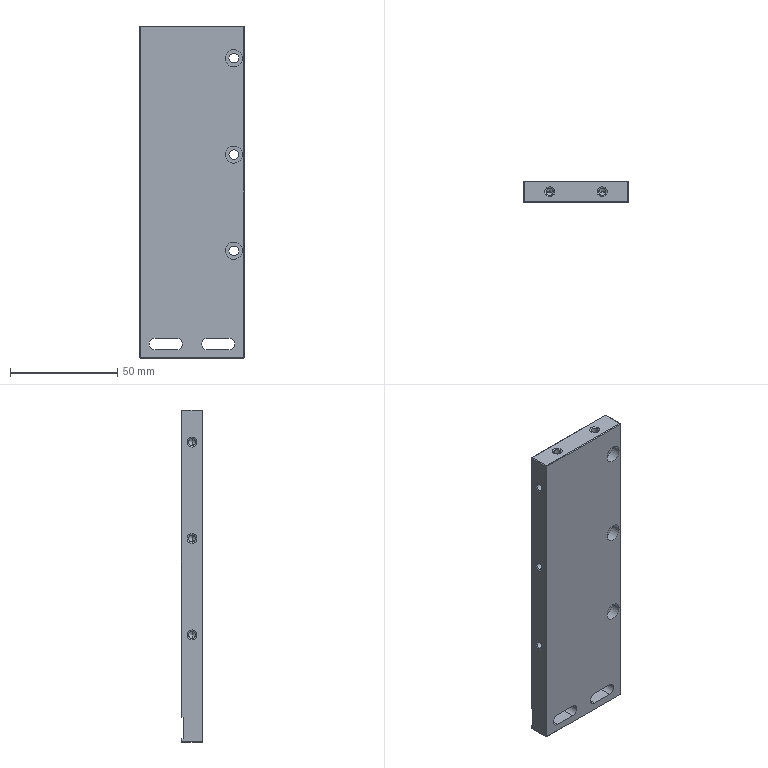Part | NX | 1 solid | 89 faces | box 49 x 10 x 155 mm | volume 72521 mm3 | cylinder 38 | plane 31 | cone 20 | commonest cylinder face diameters 3.3 x20 4.5 x6 5.5 x6 8 x6